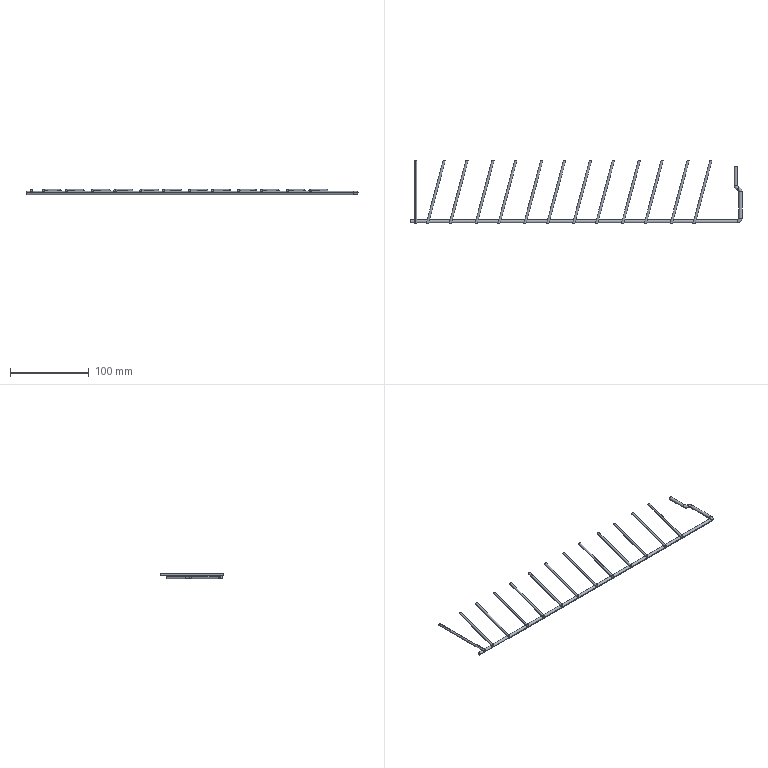Part | STEP file | ZXW722-L-178-D_23_1_1 | 1 solid | 68 faces | box 421.95 x 80.725 x 6.4 mm | volume 12477 mm3 | cylinder 34 | plane 28 | torus 6 | commonest cylinder face diameters 2.8 x26 3.9 x8